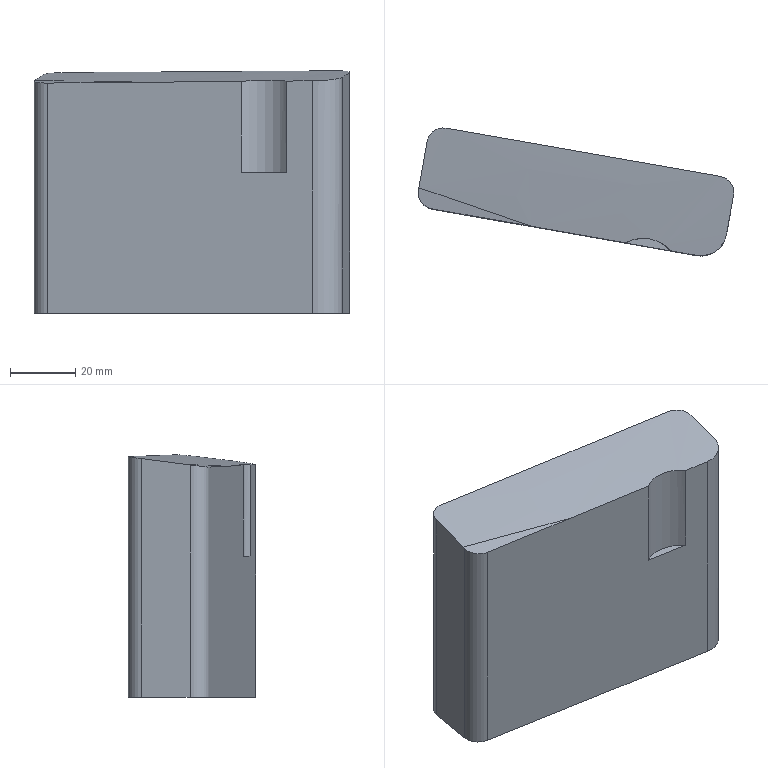Part | STEP file | gslz 2016.10.28-13_id1422_x_t | 1 solid | 13 faces | box 96.313 x 39.023 x 74.019 mm | volume 168785 mm3 | plane 6 | cylinder 5 | spline 2 | commonest cylinder face diameters 10 x3 16 x1 22 x1